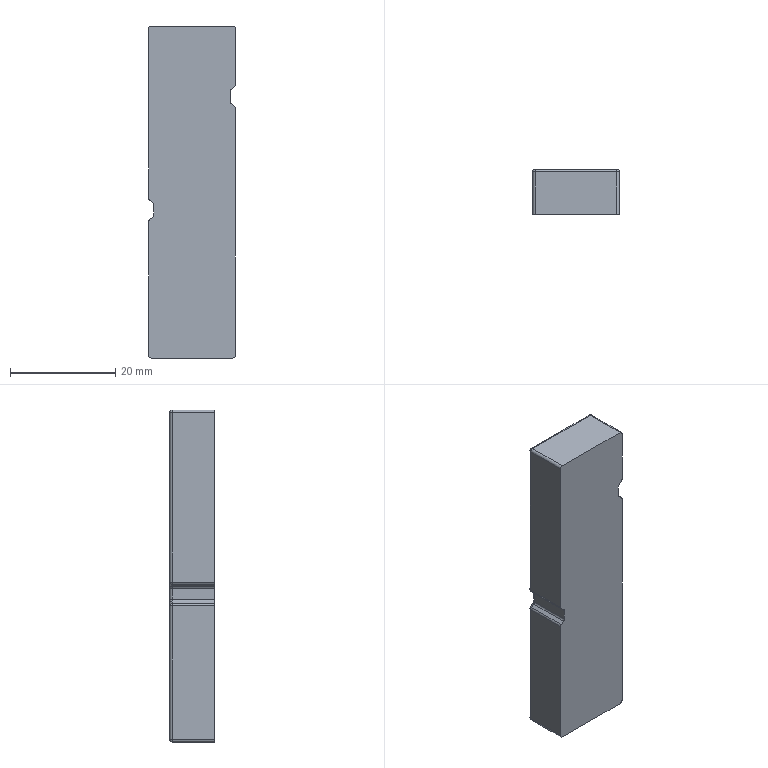Part | STEP file | SS5V1-16S3AD-08B-N1_Exhaust Cap | 1 solid | 62 faces | box 16.5 x 8.5 x 63 mm | volume 8670 mm3 | cylinder 32 | plane 16 | sphere 10 | torus 4 | commonest cylinder face diameters 1 x24 5 x4 6.15 x4